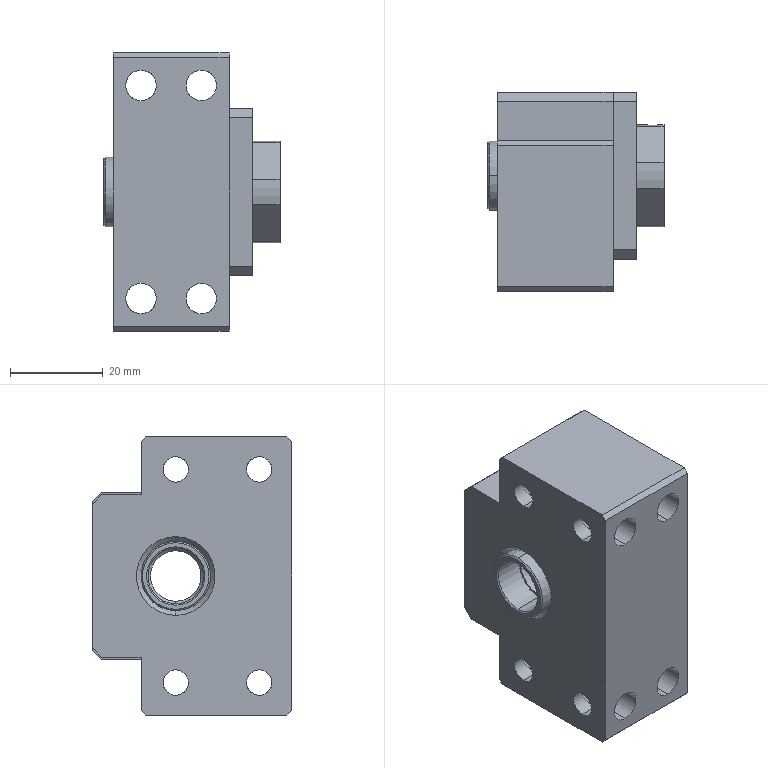Part | SolidWorks | features BaseBody 9 | 9 solids | 326 faces | box 38 x 43 x 60 mm | volume 55106 mm3 | plane 145 | cylinder 125 | cone 56 | commonest cylinder face diameters 5.5 x32 2.459 x10 3 x8 3.5 x8 6.6 x8 7 x8